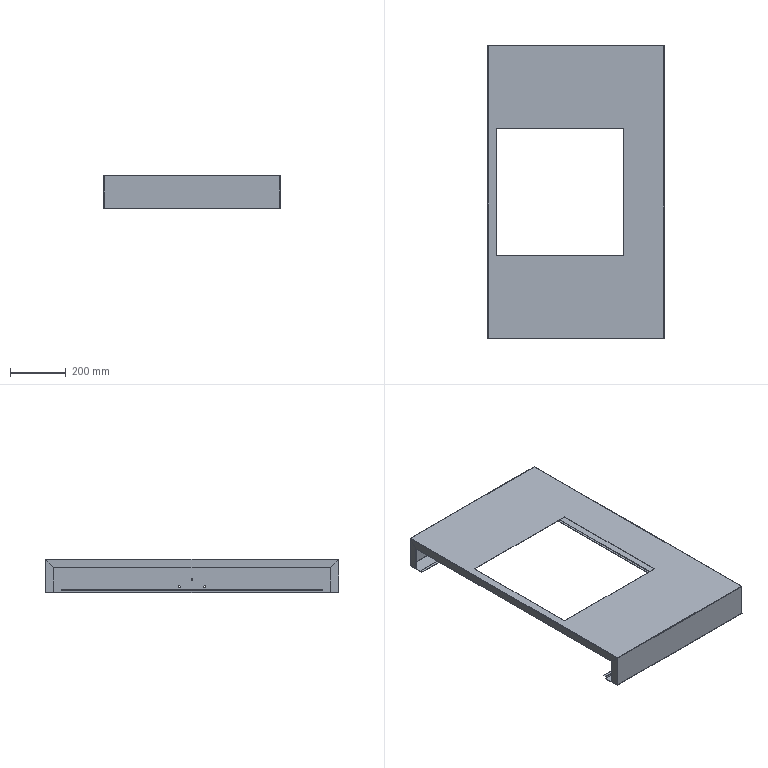Part | STEP file | HESS-408-70-15W-W-32-upper door right frame | 1 solid | 136 faces | box 630 x 1050 x 120 mm | volume 1382847 mm3 | plane 84 | cylinder 36 | spline 16 | commonest cylinder face diameters 0.2 x15 3.2 x15 6 x6